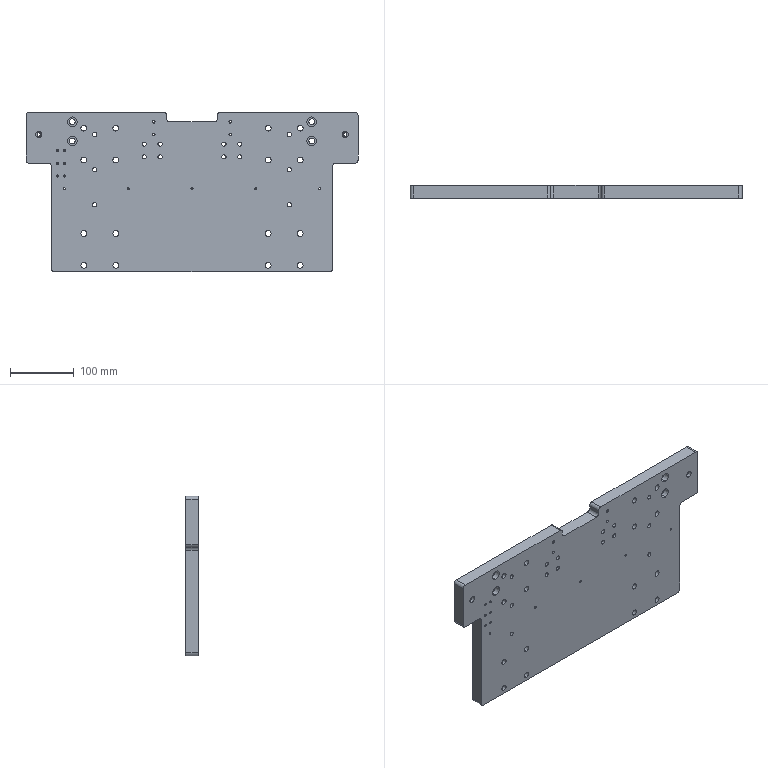Part | STEP file | Slider fixing plate | 1 solid | 236 faces | box 520 x 20 x 250 mm | volume 2234744 mm3 | cylinder 178 | plane 46 | cone 12 | commonest cylinder face diameters 9 x40 15 x40 3.3 x22 6.6 x16 10 x16 11 x16